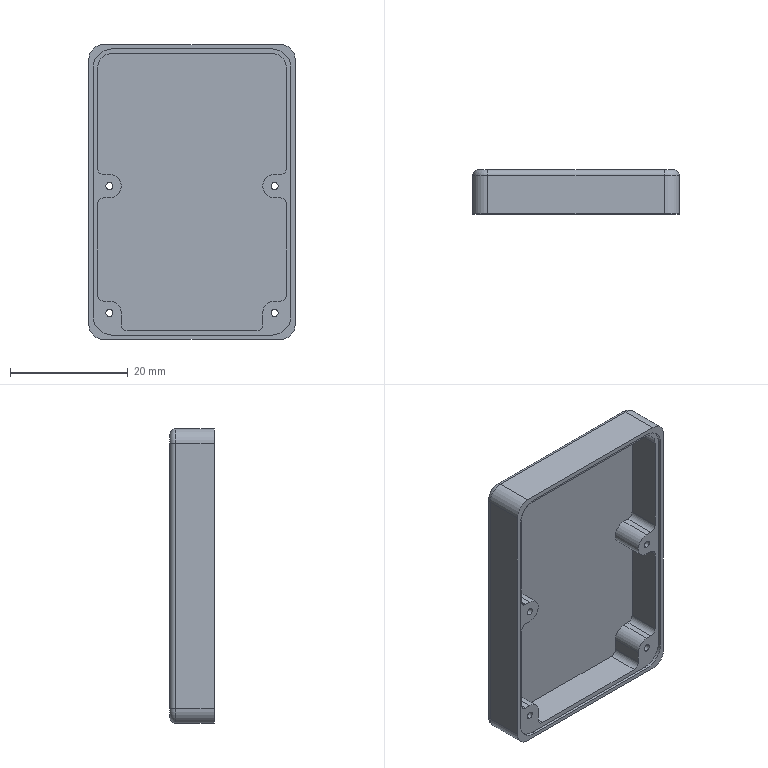Part | SolidWorks | features ICE 5, Fillet 2, Extrusion 1, Scale 1 | 1 solid | 84 faces | box 35 x 7.5 x 50 mm | volume 4265 mm3 | cylinder 42 | plane 30 | torus 12 | commonest cylinder face diameters 2 x12 1.2 x8 2.1 x8 5 x6 4 x4 6.55 x4